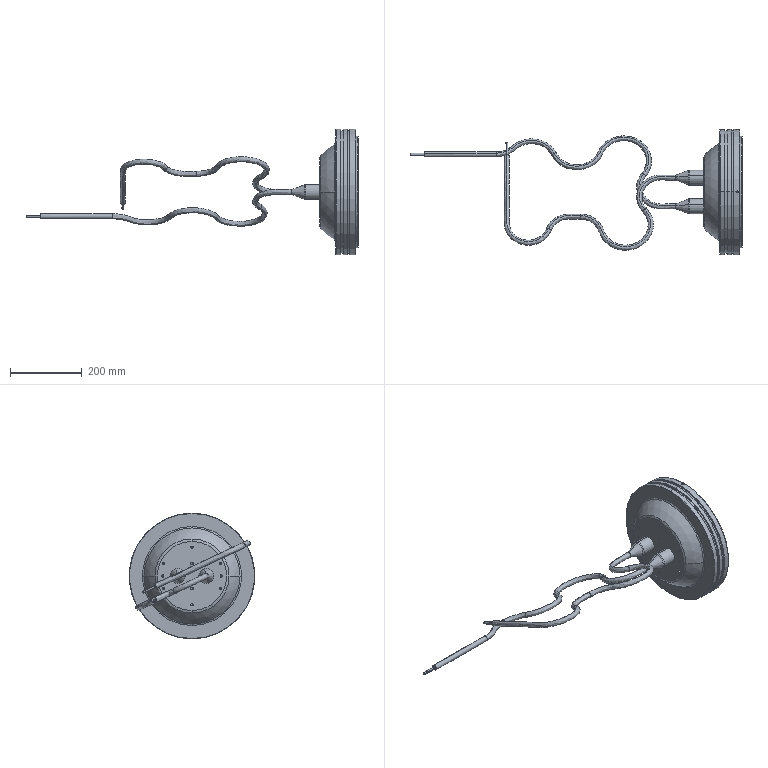Part | NX | features BREP 7 | 8 solids | 717 faces | box 924 x 350 x 350 mm | volume 7462728 mm3 | cylinder 247 | cone 178 | spline 131 | plane 100 | torus 59 | sphere 2 | commonest cylinder face diameters 30 x52 26 x48 1 x28 6.8 x18 4.2 x16 6.35 x11